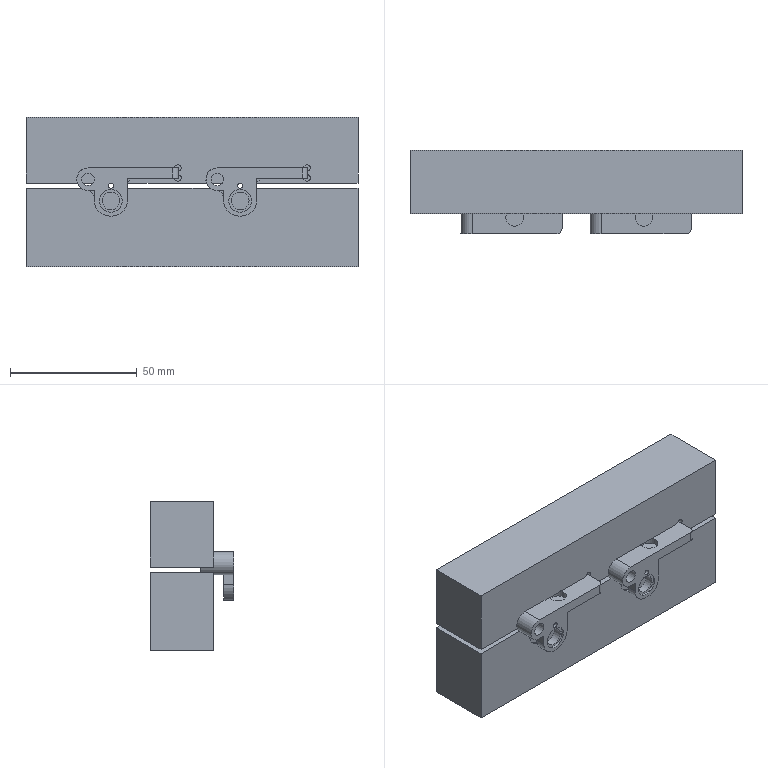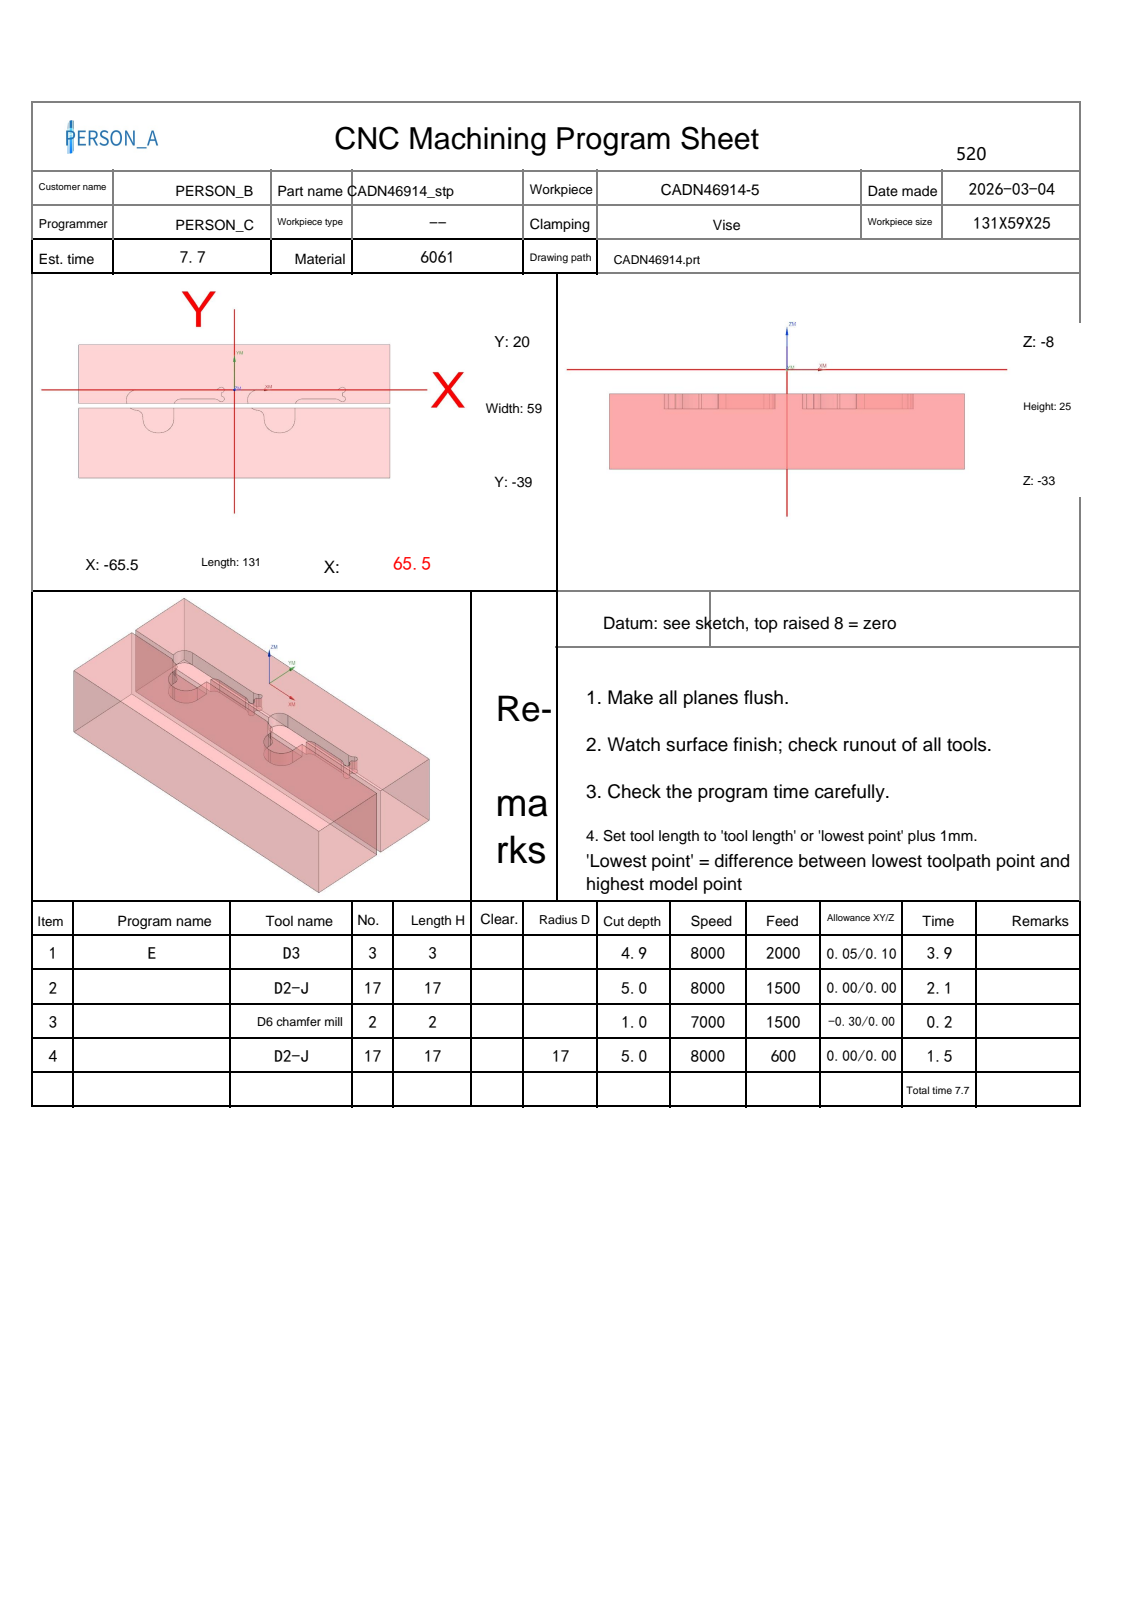NC program | NX | posted by the shop | part box 131 x 33 x 59 mm
Lines 4412 to 5424 of 10523:
N2 T17 M06
(D2-J  D=2. R=0. H=17 ce=0.00 di=0.00)
G00 G90 G54 X43.493 Y-2.917 M03 S8000
G43 H17 Z40.
M08
Z-7.9
G01 X43.492 Y-2.919 Z-7.93 F800.
Y-2.927 Z-7.958
Y-2.938 Z-7.982
Y-2.953 Z-8.004
X43.493 Y-2.971 Z-8.023
X43.496 Y-2.991 Z-8.04
X43.5 Y-3.013 Z-8.054
X43.506 Y-3.035 Z-8.066
X43.514 Y-3.058 Z-8.076
X43.524 Y-3.081 Z-8.084
X43.538 Y-3.102 Z-8.09
X43.554 Y-3.122 Z-8.095
X43.575 Y-3.139 Z-8.098
X43.599 Y-3.154 Z-8.099
X43.627 Y-3.165 Z-8.1
G02 X45.323 Y-4.176 I-1.138 J-3.835
G01 X45.5 Y-4.25
G03 X45.75 Y-4. I0.0 J.25
X45.5 Y-3.75 I-.25 J0.0
G02 X44.5 Y-2.75 I0.0 J1.
G01 Y-2.524
X44.491 Y-2.492 Z-8.101
X44.466 Y-2.471 Z-8.102
X44.428 Y-2.459 Z-8.105
X44.379 Y-2.456 Z-8.108
X44.322 Y-2.46 Z-8.112
X44.26 Y-2.472 Z-8.117
X44.195 Y-2.488 Z-8.122
X44.131 Y-2.509 Z-8.127
X44.012 Y-2.562 Z-8.138
X43.904 Y-2.63 Z-8.15
X43.807 Y-2.713 Z-8.162
X43.721 Y-2.811 Z-8.173
X43.682 Y-2.866 Z-8.178
X43.647 Y-2.922 Z-8.183
X43.619 Y-2.978 Z-8.188
X43.598 Y-3.031 Z-8.192
X43.586 Y-3.078 Z-8.195
Y-3.118 Z-8.198
X43.599 Y-3.148 Z-8.199
X43.627 Y-3.165 Z-8.2
G02 X45.323 Y-4.176 I-1.138 J-3.835
G01 X45.5 Y-4.25
G03 X45.75 Y-4. I0.0 J.25
X45.5 Y-3.75 I-.25 J0.0
G02 X44.5 Y-2.75 I0.0 J1.
G01 Y-2.524
X44.491 Y-2.492 Z-8.201
X44.466 Y-2.471 Z-8.202
X44.428 Y-2.459 Z-8.205
X44.379 Y-2.456 Z-8.208
X44.322 Y-2.46 Z-8.212
X44.26 Y-2.472 Z-8.217
X44.195 Y-2.488 Z-8.222
X44.131 Y-2.509 Z-8.227
X44.012 Y-2.562 Z-8.238
X43.904 Y-2.63 Z-8.25
X43.807 Y-2.713 Z-8.262
X43.721 Y-2.811 Z-8.273
X43.682 Y-2.866 Z-8.278
X43.647 Y-2.922 Z-8.283
X43.619 Y-2.978 Z-8.288
X43.598 Y-3.031 Z-8.292
X43.586 Y-3.078 Z-8.295
Y-3.118 Z-8.298
X43.599 Y-3.148 Z-8.299
X43.627 Y-3.165 Z-8.3
G02 X45.323 Y-4.176 I-1.138 J-3.835
G01 X45.5 Y-4.25
G03 X45.75 Y-4. I0.0 J.25
X45.5 Y-3.75 I-.25 J0.0
G02 X44.5 Y-2.75 I0.0 J1.
G01 Y-2.524
X44.491 Y-2.492 Z-8.301
X44.466 Y-2.471 Z-8.302
X44.428 Y-2.459 Z-8.305
X44.379 Y-2.456 Z-8.308
X44.322 Y-2.46 Z-8.312
X44.26 Y-2.472 Z-8.317
X44.195 Y-2.488 Z-8.322
X44.131 Y-2.509 Z-8.327
X44.012 Y-2.562 Z-8.338
X43.904 Y-2.63 Z-8.35
X43.807 Y-2.713 Z-8.362
X43.721 Y-2.811 Z-8.373
X43.682 Y-2.866 Z-8.378
X43.647 Y-2.922 Z-8.383
X43.619 Y-2.978 Z-8.388
X43.598 Y-3.031 Z-8.392
X43.586 Y-3.078 Z-8.395
Y-3.118 Z-8.398
X43.599 Y-3.148 Z-8.399
X43.627 Y-3.165 Z-8.4
G02 X45.323 Y-4.176 I-1.138 J-3.835
G01 X45.5 Y-4.25
G03 X45.75 Y-4. I0.0 J.25
X45.5 Y-3.75 I-.25 J0.0
G02 X44.5 Y-2.75 I0.0 J1.
G01 Y-2.524
X44.491 Y-2.492 Z-8.401
X44.466 Y-2.471 Z-8.402
X44.428 Y-2.459 Z-8.405
X44.379 Y-2.456 Z-8.408
X44.322 Y-2.46 Z-8.412
X44.26 Y-2.472 Z-8.417
X44.195 Y-2.488 Z-8.422
X44.131 Y-2.509 Z-8.427
X44.012 Y-2.562 Z-8.438
X43.904 Y-2.63 Z-8.45
X43.807 Y-2.713 Z-8.462
X43.721 Y-2.811 Z-8.473
X43.682 Y-2.866 Z-8.478
X43.647 Y-2.922 Z-8.483
X43.619 Y-2.978 Z-8.488
X43.598 Y-3.031 Z-8.492
X43.586 Y-3.078 Z-8.495
Y-3.118 Z-8.498
X43.599 Y-3.148 Z-8.499
X43.627 Y-3.165 Z-8.5
G02 X45.323 Y-4.176 I-1.138 J-3.835
G01 X45.5 Y-4.25
G03 X45.75 Y-4. I0.0 J.25
X45.5 Y-3.75 I-.25 J0.0
G02 X44.5 Y-2.75 I0.0 J1.
G01 Y-2.524
X44.491 Y-2.492 Z-8.501
X44.466 Y-2.471 Z-8.502
X44.428 Y-2.459 Z-8.505
X44.379 Y-2.456 Z-8.508
X44.322 Y-2.46 Z-8.512
X44.26 Y-2.472 Z-8.517
X44.195 Y-2.488 Z-8.522
X44.131 Y-2.509 Z-8.527
X44.012 Y-2.562 Z-8.538
X43.904 Y-2.63 Z-8.55
X43.807 Y-2.713 Z-8.562
X43.721 Y-2.811 Z-8.573
X43.682 Y-2.866 Z-8.578
X43.647 Y-2.922 Z-8.583
X43.619 Y-2.978 Z-8.588
X43.598 Y-3.031 Z-8.592
X43.586 Y-3.078 Z-8.595
Y-3.118 Z-8.598
X43.599 Y-3.148 Z-8.599
X43.627 Y-3.165 Z-8.6
G02 X45.323 Y-4.176 I-1.138 J-3.835
G01 X45.5 Y-4.25
G03 X45.75 Y-4. I0.0 J.25
X45.5 Y-3.75 I-.25 J0.0
G02 X44.5 Y-2.75 I0.0 J1.
G01 Y-2.524
X44.491 Y-2.492 Z-8.601
X44.466 Y-2.471 Z-8.602
X44.428 Y-2.459 Z-8.605
X44.379 Y-2.456 Z-8.608
X44.322 Y-2.46 Z-8.612
X44.26 Y-2.472 Z-8.617
X44.195 Y-2.488 Z-8.622
X44.131 Y-2.509 Z-8.627
X44.012 Y-2.562 Z-8.638
X43.904 Y-2.63 Z-8.65
X43.807 Y-2.713 Z-8.662
X43.721 Y-2.811 Z-8.673
X43.682 Y-2.866 Z-8.678
X43.647 Y-2.922 Z-8.683
X43.619 Y-2.978 Z-8.688
X43.598 Y-3.031 Z-8.692
X43.586 Y-3.078 Z-8.695
Y-3.118 Z-8.698
X43.599 Y-3.148 Z-8.699
X43.627 Y-3.165 Z-8.7
G02 X45.323 Y-4.176 I-1.138 J-3.835
G01 X45.5 Y-4.25
G03 X45.75 Y-4. I0.0 J.25
X45.5 Y-3.75 I-.25 J0.0
G02 X44.5 Y-2.75 I0.0 J1.
G01 Y-2.524
X44.491 Y-2.492 Z-8.701
X44.466 Y-2.471 Z-8.702
X44.428 Y-2.459 Z-8.705
X44.379 Y-2.456 Z-8.708
X44.322 Y-2.46 Z-8.712
X44.26 Y-2.472 Z-8.717
X44.195 Y-2.488 Z-8.722
X44.131 Y-2.509 Z-8.727
X44.012 Y-2.562 Z-8.738
X43.904 Y-2.63 Z-8.75
X43.807 Y-2.713 Z-8.762
X43.721 Y-2.811 Z-8.773
X43.682 Y-2.866 Z-8.778
X43.647 Y-2.922 Z-8.783
X43.619 Y-2.978 Z-8.788
X43.598 Y-3.031 Z-8.792
X43.586 Y-3.078 Z-8.795
Y-3.118 Z-8.798
X43.599 Y-3.148 Z-8.799
X43.627 Y-3.165 Z-8.8
G02 X45.323 Y-4.176 I-1.138 J-3.835
G01 X45.5 Y-4.25
G03 X45.75 Y-4. I0.0 J.25
X45.5 Y-3.75 I-.25 J0.0
G02 X44.5 Y-2.75 I0.0 J1.
G01 Y-2.524
X44.491 Y-2.492 Z-8.801
X44.466 Y-2.471 Z-8.802
X44.428 Y-2.459 Z-8.805
X44.379 Y-2.456 Z-8.808
X44.322 Y-2.46 Z-8.812
X44.26 Y-2.472 Z-8.817
X44.195 Y-2.488 Z-8.822
X44.131 Y-2.509 Z-8.827
X44.012 Y-2.562 Z-8.838
X43.904 Y-2.63 Z-8.85
X43.807 Y-2.713 Z-8.862
X43.721 Y-2.811 Z-8.873
X43.682 Y-2.866 Z-8.878
X43.647 Y-2.922 Z-8.883
X43.619 Y-2.978 Z-8.888
X43.598 Y-3.031 Z-8.892
X43.586 Y-3.078 Z-8.895
Y-3.118 Z-8.898
X43.599 Y-3.148 Z-8.899
X43.627 Y-3.165 Z-8.9
G02 X45.323 Y-4.176 I-1.138 J-3.835
G01 X45.5 Y-4.25
G03 X45.75 Y-4. I0.0 J.25
X45.5 Y-3.75 I-.25 J0.0
G02 X44.5 Y-2.75 I0.0 J1.
G01 Y-2.524
X44.491 Y-2.492 Z-8.901
X44.466 Y-2.471 Z-8.902
X44.428 Y-2.459 Z-8.905
X44.379 Y-2.456 Z-8.908
X44.322 Y-2.46 Z-8.912
X44.26 Y-2.472 Z-8.917
X44.195 Y-2.488 Z-8.922
X44.131 Y-2.509 Z-8.927
X44.012 Y-2.562 Z-8.938
X43.904 Y-2.63 Z-8.95
X43.807 Y-2.713 Z-8.962
X43.721 Y-2.811 Z-8.973
X43.682 Y-2.866 Z-8.978
X43.647 Y-2.922 Z-8.983
X43.619 Y-2.978 Z-8.988
X43.598 Y-3.031 Z-8.992
X43.586 Y-3.078 Z-8.995
Y-3.118 Z-8.998
X43.599 Y-3.148 Z-8.999
X43.627 Y-3.165 Z-9.
G02 X45.323 Y-4.176 I-1.138 J-3.835
G01 X45.5 Y-4.25
G03 X45.75 Y-4. I0.0 J.25
X45.5 Y-3.75 I-.25 J0.0
G02 X44.5 Y-2.75 I0.0 J1.
G01 Y-2.524
X44.491 Y-2.492 Z-9.001
X44.466 Y-2.471 Z-9.002
X44.428 Y-2.459 Z-9.005
X44.379 Y-2.456 Z-9.008
X44.322 Y-2.46 Z-9.012
X44.26 Y-2.472 Z-9.017
X44.195 Y-2.488 Z-9.022
X44.131 Y-2.509 Z-9.027
X44.012 Y-2.562 Z-9.038
X43.904 Y-2.63 Z-9.05
X43.807 Y-2.713 Z-9.062
X43.721 Y-2.811 Z-9.073
X43.682 Y-2.866 Z-9.078
X43.647 Y-2.922 Z-9.083
X43.619 Y-2.978 Z-9.088
X43.598 Y-3.031 Z-9.092
X43.586 Y-3.078 Z-9.095
Y-3.118 Z-9.098
X43.599 Y-3.148 Z-9.099
X43.627 Y-3.165 Z-9.1
G02 X45.323 Y-4.176 I-1.138 J-3.835
G01 X45.5 Y-4.25
G03 X45.75 Y-4. I0.0 J.25
X45.5 Y-3.75 I-.25 J0.0
G02 X44.5 Y-2.75 I0.0 J1.
G01 Y-2.524
X44.491 Y-2.492 Z-9.101
X44.466 Y-2.471 Z-9.102
X44.428 Y-2.459 Z-9.105
X44.379 Y-2.456 Z-9.108
X44.322 Y-2.46 Z-9.112
X44.26 Y-2.472 Z-9.117
X44.195 Y-2.488 Z-9.122
X44.131 Y-2.509 Z-9.127
X44.012 Y-2.562 Z-9.138
X43.904 Y-2.63 Z-9.15
X43.807 Y-2.713 Z-9.162
X43.721 Y-2.811 Z-9.173
X43.682 Y-2.866 Z-9.178
X43.647 Y-2.922 Z-9.183
X43.619 Y-2.978 Z-9.188
X43.598 Y-3.031 Z-9.192
X43.586 Y-3.078 Z-9.195
Y-3.118 Z-9.198
X43.599 Y-3.148 Z-9.199
X43.627 Y-3.165 Z-9.2
G02 X45.323 Y-4.176 I-1.138 J-3.835
G01 X45.5 Y-4.25
G03 X45.75 Y-4. I0.0 J.25
X45.5 Y-3.75 I-.25 J0.0
G02 X44.5 Y-2.75 I0.0 J1.
G01 Y-2.524
X44.491 Y-2.492 Z-9.201
X44.466 Y-2.471 Z-9.202
X44.428 Y-2.459 Z-9.205
X44.379 Y-2.456 Z-9.208
X44.322 Y-2.46 Z-9.212
X44.26 Y-2.472 Z-9.217
X44.195 Y-2.488 Z-9.222
X44.131 Y-2.509 Z-9.227
X44.012 Y-2.562 Z-9.238
X43.904 Y-2.63 Z-9.25
X43.807 Y-2.713 Z-9.262
X43.721 Y-2.811 Z-9.273
X43.682 Y-2.866 Z-9.278
X43.647 Y-2.922 Z-9.283
X43.619 Y-2.978 Z-9.288
X43.598 Y-3.031 Z-9.292
X43.586 Y-3.078 Z-9.295
Y-3.118 Z-9.298
X43.599 Y-3.148 Z-9.299
X43.627 Y-3.165 Z-9.3
G02 X45.323 Y-4.176 I-1.138 J-3.835
G01 X45.5 Y-4.25
G03 X45.75 Y-4. I0.0 J.25
X45.5 Y-3.75 I-.25 J0.0
G02 X44.5 Y-2.75 I0.0 J1.
G01 Y-2.524
X44.491 Y-2.492 Z-9.301
X44.466 Y-2.471 Z-9.302
X44.428 Y-2.459 Z-9.305
X44.379 Y-2.456 Z-9.308
X44.322 Y-2.46 Z-9.312
X44.26 Y-2.472 Z-9.317
X44.195 Y-2.488 Z-9.322
X44.131 Y-2.509 Z-9.327
X44.012 Y-2.562 Z-9.338
X43.904 Y-2.63 Z-9.35
X43.807 Y-2.713 Z-9.362
X43.721 Y-2.811 Z-9.373
X43.682 Y-2.866 Z-9.378
X43.647 Y-2.922 Z-9.383
X43.619 Y-2.978 Z-9.388
X43.598 Y-3.031 Z-9.392
X43.586 Y-3.078 Z-9.395
Y-3.118 Z-9.398
X43.599 Y-3.148 Z-9.399
X43.627 Y-3.165 Z-9.4
G02 X45.323 Y-4.176 I-1.138 J-3.835
G01 X45.5 Y-4.25
G03 X45.75 Y-4. I0.0 J.25
X45.5 Y-3.75 I-.25 J0.0
G02 X44.5 Y-2.75 I0.0 J1.
G01 Y-2.524
X44.491 Y-2.492 Z-9.401
X44.466 Y-2.471 Z-9.402
X44.428 Y-2.459 Z-9.405
X44.379 Y-2.456 Z-9.408
X44.322 Y-2.46 Z-9.412
X44.26 Y-2.472 Z-9.417
X44.195 Y-2.488 Z-9.422
X44.131 Y-2.509 Z-9.427
X44.012 Y-2.562 Z-9.438
X43.904 Y-2.63 Z-9.45
X43.807 Y-2.713 Z-9.462
X43.721 Y-2.811 Z-9.473
X43.682 Y-2.866 Z-9.478
X43.647 Y-2.922 Z-9.483
X43.619 Y-2.978 Z-9.488
X43.598 Y-3.031 Z-9.492
X43.586 Y-3.078 Z-9.495
Y-3.118 Z-9.498
X43.599 Y-3.148 Z-9.499
X43.627 Y-3.165 Z-9.5
G02 X45.323 Y-4.176 I-1.138 J-3.835
G01 X45.5 Y-4.25
G03 X45.75 Y-4. I0.0 J.25
X45.5 Y-3.75 I-.25 J0.0
G02 X44.5 Y-2.75 I0.0 J1.
G01 Y-2.524
X44.491 Y-2.492 Z-9.501
X44.466 Y-2.471 Z-9.502
X44.428 Y-2.459 Z-9.505
X44.379 Y-2.456 Z-9.508
X44.322 Y-2.46 Z-9.512
X44.26 Y-2.472 Z-9.517
X44.195 Y-2.488 Z-9.522
X44.131 Y-2.509 Z-9.527
X44.012 Y-2.562 Z-9.538
X43.904 Y-2.63 Z-9.55
X43.807 Y-2.713 Z-9.562
X43.721 Y-2.811 Z-9.573
X43.682 Y-2.866 Z-9.578
X43.647 Y-2.922 Z-9.583
X43.619 Y-2.978 Z-9.588
X43.598 Y-3.031 Z-9.592
X43.586 Y-3.078 Z-9.595
Y-3.118 Z-9.598
X43.599 Y-3.148 Z-9.599
X43.627 Y-3.165 Z-9.6
G02 X45.323 Y-4.176 I-1.138 J-3.835
G01 X45.5 Y-4.25
G03 X45.75 Y-4. I0.0 J.25
X45.5 Y-3.75 I-.25 J0.0
G02 X44.5 Y-2.75 I0.0 J1.
G01 Y-2.524
X44.491 Y-2.492 Z-9.601
X44.466 Y-2.471 Z-9.602
X44.428 Y-2.459 Z-9.605
X44.379 Y-2.456 Z-9.608
X44.322 Y-2.46 Z-9.612
X44.26 Y-2.472 Z-9.617
X44.195 Y-2.488 Z-9.622
X44.131 Y-2.509 Z-9.627
X44.012 Y-2.562 Z-9.638
X43.904 Y-2.63 Z-9.65
X43.807 Y-2.713 Z-9.662
X43.721 Y-2.811 Z-9.673
X43.682 Y-2.866 Z-9.678
X43.647 Y-2.922 Z-9.683
X43.619 Y-2.978 Z-9.688
X43.598 Y-3.031 Z-9.692
X43.586 Y-3.078 Z-9.695
Y-3.118 Z-9.698
X43.599 Y-3.148 Z-9.699
X43.627 Y-3.165 Z-9.7
G02 X45.323 Y-4.176 I-1.138 J-3.835
G01 X45.5 Y-4.25
G03 X45.75 Y-4. I0.0 J.25
X45.5 Y-3.75 I-.25 J0.0
G02 X44.5 Y-2.75 I0.0 J1.
G01 Y-2.524
X44.491 Y-2.492 Z-9.701
X44.466 Y-2.471 Z-9.702
X44.428 Y-2.459 Z-9.705
X44.379 Y-2.456 Z-9.708
X44.322 Y-2.46 Z-9.712
X44.26 Y-2.472 Z-9.717
X44.195 Y-2.488 Z-9.722
X44.131 Y-2.509 Z-9.727
X44.012 Y-2.562 Z-9.738
X43.904 Y-2.63 Z-9.75
X43.807 Y-2.713 Z-9.762
X43.721 Y-2.811 Z-9.773
X43.682 Y-2.866 Z-9.778
X43.647 Y-2.922 Z-9.783
X43.619 Y-2.978 Z-9.788
X43.598 Y-3.031 Z-9.792
X43.586 Y-3.078 Z-9.795
Y-3.118 Z-9.798
X43.599 Y-3.148 Z-9.799
X43.627 Y-3.165 Z-9.8
G02 X45.323 Y-4.176 I-1.138 J-3.835
G01 X45.5 Y-4.25
G03 X45.75 Y-4. I0.0 J.25
X45.5 Y-3.75 I-.25 J0.0
G02 X44.5 Y-2.75 I0.0 J1.
G01 Y-2.524
X44.491 Y-2.492 Z-9.801
X44.466 Y-2.471 Z-9.802
X44.428 Y-2.459 Z-9.805
X44.379 Y-2.456 Z-9.808
X44.322 Y-2.46 Z-9.812
X44.26 Y-2.472 Z-9.817
X44.195 Y-2.488 Z-9.822
X44.131 Y-2.509 Z-9.827
X44.012 Y-2.562 Z-9.838
X43.904 Y-2.63 Z-9.85
X43.807 Y-2.713 Z-9.862
X43.721 Y-2.811 Z-9.873
X43.682 Y-2.866 Z-9.878
X43.647 Y-2.922 Z-9.883
X43.619 Y-2.978 Z-9.888
X43.598 Y-3.031 Z-9.892
X43.586 Y-3.078 Z-9.895
Y-3.118 Z-9.898
X43.599 Y-3.148 Z-9.899
X43.627 Y-3.165 Z-9.9
G02 X45.323 Y-4.176 I-1.138 J-3.835
G01 X45.5 Y-4.25
G03 X45.75 Y-4. I0.0 J.25
X45.5 Y-3.75 I-.25 J0.0
G02 X44.5 Y-2.75 I0.0 J1.
G01 Y-2.524
X44.491 Y-2.492 Z-9.901
X44.466 Y-2.471 Z-9.902
X44.428 Y-2.459 Z-9.905
X44.379 Y-2.456 Z-9.908
X44.322 Y-2.46 Z-9.912
X44.26 Y-2.472 Z-9.917
X44.195 Y-2.488 Z-9.922
X44.131 Y-2.509 Z-9.927
X44.012 Y-2.562 Z-9.938
X43.904 Y-2.63 Z-9.95
X43.807 Y-2.713 Z-9.962
X43.721 Y-2.811 Z-9.973
X43.682 Y-2.866 Z-9.978
X43.647 Y-2.922 Z-9.983
X43.619 Y-2.978 Z-9.988
X43.598 Y-3.031 Z-9.992
X43.586 Y-3.078 Z-9.995
Y-3.118 Z-9.998
X43.599 Y-3.148 Z-9.999
X43.627 Y-3.165 Z-10.
G02 X45.323 Y-4.176 I-1.138 J-3.835
G01 X45.5 Y-4.25
G03 X45.75 Y-4. I0.0 J.25
X45.5 Y-3.75 I-.25 J0.0
G02 X44.5 Y-2.75 I0.0 J1.
G01 Y-2.524
X44.491 Y-2.492 Z-10.001
X44.466 Y-2.471 Z-10.002
X44.428 Y-2.459 Z-10.005
X44.379 Y-2.456 Z-10.008
X44.322 Y-2.46 Z-10.012
X44.26 Y-2.472 Z-10.017
X44.195 Y-2.488 Z-10.022
X44.131 Y-2.509 Z-10.027
X44.012 Y-2.562 Z-10.038
X43.904 Y-2.63 Z-10.05
X43.807 Y-2.713 Z-10.062
X43.721 Y-2.811 Z-10.073
X43.682 Y-2.866 Z-10.078
X43.647 Y-2.922 Z-10.083
X43.619 Y-2.978 Z-10.088
X43.598 Y-3.031 Z-10.092
X43.586 Y-3.078 Z-10.095
Y-3.118 Z-10.098
X43.599 Y-3.148 Z-10.099
X43.627 Y-3.165 Z-10.1
G02 X45.323 Y-4.176 I-1.138 J-3.835
G01 X45.5 Y-4.25
G03 X45.75 Y-4. I0.0 J.25
X45.5 Y-3.75 I-.25 J0.0
G02 X44.5 Y-2.75 I0.0 J1.
G01 Y-2.524
X44.491 Y-2.492 Z-10.101
X44.466 Y-2.471 Z-10.102
X44.428 Y-2.459 Z-10.105
X44.379 Y-2.456 Z-10.108
X44.322 Y-2.46 Z-10.112
X44.26 Y-2.472 Z-10.117
X44.195 Y-2.488 Z-10.122
X44.131 Y-2.509 Z-10.127
X44.012 Y-2.562 Z-10.138
X43.904 Y-2.63 Z-10.15
X43.807 Y-2.713 Z-10.162
X43.721 Y-2.811 Z-10.173
X43.682 Y-2.866 Z-10.178
X43.647 Y-2.922 Z-10.183
X43.619 Y-2.978 Z-10.188
X43.598 Y-3.031 Z-10.192
X43.586 Y-3.078 Z-10.195
Y-3.118 Z-10.198
X43.599 Y-3.148 Z-10.199
X43.627 Y-3.165 Z-10.2
G02 X45.323 Y-4.176 I-1.138 J-3.835
G01 X45.5 Y-4.25
G03 X45.75 Y-4. I0.0 J.25
X45.5 Y-3.75 I-.25 J0.0
G02 X44.5 Y-2.75 I0.0 J1.
G01 Y-2.524
X44.491 Y-2.492 Z-10.201
X44.466 Y-2.471 Z-10.202
X44.428 Y-2.459 Z-10.205
X44.379 Y-2.456 Z-10.208
X44.322 Y-2.46 Z-10.212
X44.26 Y-2.472 Z-10.217
X44.195 Y-2.488 Z-10.222
X44.131 Y-2.509 Z-10.227
X44.012 Y-2.562 Z-10.238
X43.904 Y-2.63 Z-10.25
X43.807 Y-2.713 Z-10.262
X43.721 Y-2.811 Z-10.273
X43.682 Y-2.866 Z-10.278
X43.647 Y-2.922 Z-10.283
X43.619 Y-2.978 Z-10.288
X43.598 Y-3.031 Z-10.292
X43.586 Y-3.078 Z-10.295
Y-3.118 Z-10.298
X43.599 Y-3.148 Z-10.299
X43.627 Y-3.165 Z-10.3
G02 X45.323 Y-4.176 I-1.138 J-3.835
G01 X45.5 Y-4.25
G03 X45.75 Y-4. I0.0 J.25
X45.5 Y-3.75 I-.25 J0.0
G02 X44.5 Y-2.75 I0.0 J1.
G01 Y-2.524
X44.491 Y-2.492 Z-10.301
X44.466 Y-2.471 Z-10.302
X44.428 Y-2.459 Z-10.305
X44.379 Y-2.456 Z-10.308
X44.322 Y-2.46 Z-10.312
X44.26 Y-2.472 Z-10.317
X44.195 Y-2.488 Z-10.322
X44.131 Y-2.509 Z-10.327
X44.012 Y-2.562 Z-10.338
X43.904 Y-2.63 Z-10.35
X43.807 Y-2.713 Z-10.362
X43.721 Y-2.811 Z-10.373
X43.682 Y-2.866 Z-10.378
X43.647 Y-2.922 Z-10.383
X43.619 Y-2.978 Z-10.388
X43.598 Y-3.031 Z-10.392
X43.586 Y-3.078 Z-10.395
Y-3.118 Z-10.398
X43.599 Y-3.148 Z-10.399
X43.627 Y-3.165 Z-10.4
G02 X45.323 Y-4.176 I-1.138 J-3.835
G01 X45.5 Y-4.25
G03 X45.75 Y-4. I0.0 J.25
X45.5 Y-3.75 I-.25 J0.0
G02 X44.5 Y-2.75 I0.0 J1.
G01 Y-2.524
X44.491 Y-2.492 Z-10.401
X44.466 Y-2.471 Z-10.402
X44.428 Y-2.459 Z-10.405
X44.379 Y-2.456 Z-10.408
X44.322 Y-2.46 Z-10.412
X44.26 Y-2.472 Z-10.417
X44.195 Y-2.488 Z-10.422
X44.131 Y-2.509 Z-10.427
X44.012 Y-2.562 Z-10.438
X43.904 Y-2.63 Z-10.45
X43.807 Y-2.713 Z-10.462
X43.721 Y-2.811 Z-10.473
X43.682 Y-2.866 Z-10.478
X43.647 Y-2.922 Z-10.483
X43.619 Y-2.978 Z-10.488
X43.598 Y-3.031 Z-10.492
X43.586 Y-3.078 Z-10.495
Y-3.118 Z-10.498
X43.599 Y-3.148 Z-10.499
X43.627 Y-3.165 Z-10.5
G02 X45.323 Y-4.176 I-1.138 J-3.835
G01 X45.5 Y-4.25
G03 X45.75 Y-4. I0.0 J.25
X45.5 Y-3.75 I-.25 J0.0
G02 X44.5 Y-2.75 I0.0 J1.
G01 Y-2.524
X44.491 Y-2.492 Z-10.501
X44.466 Y-2.471 Z-10.502
X44.428 Y-2.459 Z-10.505
X44.379 Y-2.456 Z-10.508
X44.322 Y-2.46 Z-10.512
X44.26 Y-2.472 Z-10.517
X44.195 Y-2.488 Z-10.522
X44.131 Y-2.509 Z-10.527
X44.012 Y-2.562 Z-10.538
X43.904 Y-2.63 Z-10.55
X43.807 Y-2.713 Z-10.562
X43.721 Y-2.811 Z-10.573
X43.682 Y-2.866 Z-10.578
X43.647 Y-2.922 Z-10.583
X43.619 Y-2.978 Z-10.588
X43.598 Y-3.031 Z-10.592
X43.586 Y-3.078 Z-10.595
Y-3.118 Z-10.598
X43.599 Y-3.148 Z-10.599
X43.627 Y-3.165 Z-10.6
G02 X45.323 Y-4.176 I-1.138 J-3.835
G01 X45.5 Y-4.25
G03 X45.75 Y-4. I0.0 J.25
X45.5 Y-3.75 I-.25 J0.0
G02 X44.5 Y-2.75 I0.0 J1.
G01 Y-2.524
X44.491 Y-2.492 Z-10.601
X44.466 Y-2.471 Z-10.602
X44.428 Y-2.459 Z-10.605
X44.379 Y-2.456 Z-10.608
X44.322 Y-2.46 Z-10.612
X44.26 Y-2.472 Z-10.617
X44.195 Y-2.488 Z-10.622
X44.131 Y-2.509 Z-10.627
X44.012 Y-2.562 Z-10.638
X43.904 Y-2.63 Z-10.65
X43.807 Y-2.713 Z-10.662
X43.721 Y-2.811 Z-10.673
X43.682 Y-2.866 Z-10.678
X43.647 Y-2.922 Z-10.683
X43.619 Y-2.978 Z-10.688
X43.598 Y-3.031 Z-10.692
X43.586 Y-3.078 Z-10.695
Y-3.118 Z-10.698
X43.599 Y-3.148 Z-10.699
X43.627 Y-3.165 Z-10.7
G02 X45.323 Y-4.176 I-1.138 J-3.835
G01 X45.5 Y-4.25
G03 X45.75 Y-4. I0.0 J.25
X45.5 Y-3.75 I-.25 J0.0
G02 X44.5 Y-2.75 I0.0 J1.
G01 Y-2.524
X44.491 Y-2.492 Z-10.701
X44.466 Y-2.471 Z-10.702
X44.428 Y-2.459 Z-10.705
X44.379 Y-2.456 Z-10.708
X44.322 Y-2.46 Z-10.712
X44.26 Y-2.472 Z-10.717
X44.195 Y-2.488 Z-10.722
X44.131 Y-2.509 Z-10.727
X44.012 Y-2.562 Z-10.738
X43.904 Y-2.63 Z-10.75
X43.807 Y-2.713 Z-10.762
X43.721 Y-2.811 Z-10.773
X43.682 Y-2.866 Z-10.778
X43.647 Y-2.922 Z-10.783
X43.619 Y-2.978 Z-10.788
X43.598 Y-3.031 Z-10.792
X43.586 Y-3.078 Z-10.795
Y-3.118 Z-10.798
X43.599 Y-3.148 Z-10.799
X43.627 Y-3.165 Z-10.8
G02 X45.323 Y-4.176 I-1.138 J-3.835
G01 X45.5 Y-4.25
G03 X45.75 Y-4. I0.0 J.25
X45.5 Y-3.75 I-.25 J0.0
G02 X44.5 Y-2.75 I0.0 J1.
G01 Y-2.524
X44.491 Y-2.492 Z-10.801
X44.466 Y-2.471 Z-10.802
X44.428 Y-2.459 Z-10.805
X44.379 Y-2.456 Z-10.808
X44.322 Y-2.46 Z-10.812
X44.26 Y-2.472 Z-10.817
X44.195 Y-2.488 Z-10.822
X44.131 Y-2.509 Z-10.827
X44.012 Y-2.562 Z-10.838
X43.904 Y-2.63 Z-10.85
X43.807 Y-2.713 Z-10.862
X43.721 Y-2.811 Z-10.873
X43.682 Y-2.866 Z-10.878
X43.647 Y-2.922 Z-10.883
X43.619 Y-2.978 Z-10.888
X43.598 Y-3.031 Z-10.892
X43.586 Y-3.078 Z-10.895
Y-3.118 Z-10.898
X43.599 Y-3.148 Z-10.899
X43.627 Y-3.165 Z-10.9
G02 X45.323 Y-4.176 I-1.138 J-3.835
G01 X45.5 Y-4.25
G03 X45.75 Y-4. I0.0 J.25
X45.5 Y-3.75 I-.25 J0.0
G02 X44.5 Y-2.75 I0.0 J1.
G01 Y-2.524
X44.491 Y-2.492 Z-10.901
X44.466 Y-2.471 Z-10.902
X44.428 Y-2.459 Z-10.905
X44.379 Y-2.456 Z-10.908
X44.322 Y-2.46 Z-10.912
X44.26 Y-2.472 Z-10.917
X44.195 Y-2.488 Z-10.922
X44.131 Y-2.509 Z-10.927
X44.012 Y-2.562 Z-10.938
X43.904 Y-2.63 Z-10.95
X43.807 Y-2.713 Z-10.962
X43.721 Y-2.811 Z-10.973
X43.682 Y-2.866 Z-10.978
X43.647 Y-2.922 Z-10.983
X43.619 Y-2.978 Z-10.988
X43.598 Y-3.031 Z-10.992
X43.586 Y-3.078 Z-10.995
Y-3.118 Z-10.998
X43.599 Y-3.148 Z-10.999
X43.627 Y-3.165 Z-11.
G02 X45.323 Y-4.176 I-1.138 J-3.835
G01 X45.5 Y-4.25
G03 X45.75 Y-4. I0.0 J.25
X45.5 Y-3.75 I-.25 J0.0
G02 X44.5 Y-2.75 I0.0 J1.
G01 Y-2.524
X44.491 Y-2.492 Z-11.001
X44.466 Y-2.471 Z-11.002
X44.428 Y-2.459 Z-11.005
X44.379 Y-2.456 Z-11.008
X44.322 Y-2.46 Z-11.012
X44.26 Y-2.472 Z-11.017
X44.195 Y-2.488 Z-11.022
X44.131 Y-2.509 Z-11.027
X44.012 Y-2.562 Z-11.038
X43.904 Y-2.63 Z-11.05
X43.807 Y-2.713 Z-11.062
X43.721 Y-2.811 Z-11.073
X43.682 Y-2.866 Z-11.078
X43.647 Y-2.922 Z-11.083
X43.619 Y-2.978 Z-11.088
X43.598 Y-3.031 Z-11.092
X43.586 Y-3.078 Z-11.095
Y-3.118 Z-11.098
X43.599 Y-3.148 Z-11.099
X43.627 Y-3.165 Z-11.1
G02 X45.323 Y-4.176 I-1.138 J-3.835
G01 X45.5 Y-4.25
G03 X45.75 Y-4. I0.0 J.25
X45.5 Y-3.75 I-.25 J0.0
G02 X44.5 Y-2.75 I0.0 J1.
G01 Y-2.524
X44.491 Y-2.492 Z-11.101
X44.466 Y-2.471 Z-11.102
X44.428 Y-2.459 Z-11.105
X44.379 Y-2.456 Z-11.108
X44.322 Y-2.46 Z-11.112
X44.26 Y-2.472 Z-11.117
X44.195 Y-2.488 Z-11.122
X44.131 Y-2.509 Z-11.127
X44.012 Y-2.562 Z-11.138
X43.904 Y-2.63 Z-11.15
X43.807 Y-2.713 Z-11.162
X43.721 Y-2.811 Z-11.173
X43.682 Y-2.866 Z-11.178
X43.647 Y-2.922 Z-11.183
X43.619 Y-2.978 Z-11.188
X43.598 Y-3.031 Z-11.192
X43.586 Y-3.078 Z-11.195
Y-3.118 Z-11.198
X43.599 Y-3.148 Z-11.199
X43.627 Y-3.165 Z-11.2
G02 X45.323 Y-4.176 I-1.138 J-3.835
G01 X45.5 Y-4.25
G03 X45.75 Y-4. I0.0 J.25
X45.5 Y-3.75 I-.25 J0.0
G02 X44.5 Y-2.75 I0.0 J1.
G01 Y-2.524
X44.491 Y-2.492 Z-11.201
X44.466 Y-2.471 Z-11.202
X44.428 Y-2.459 Z-11.205
X44.379 Y-2.456 Z-11.208
X44.322 Y-2.46 Z-11.212
X44.26 Y-2.472 Z-11.217
X44.195 Y-2.488 Z-11.222
X44.131 Y-2.509 Z-11.227
X44.012 Y-2.562 Z-11.238
X43.904 Y-2.63 Z-11.25
X43.807 Y-2.713 Z-11.262
X43.721 Y-2.811 Z-11.273
X43.682 Y-2.866 Z-11.278
X43.647 Y-2.922 Z-11.283
X43.619 Y-2.978 Z-11.288
X43.598 Y-3.031 Z-11.292
X43.586 Y-3.078 Z-11.295
Y-3.118 Z-11.298
X43.599 Y-3.148 Z-11.299
X43.627 Y-3.165 Z-11.3
G02 X45.323 Y-4.176 I-1.138 J-3.835
G01 X45.5 Y-4.25
G03 X45.75 Y-4. I0.0 J.25
X45.5 Y-3.75 I-.25 J0.0
G02 X44.5 Y-2.75 I0.0 J1.
G01 Y-2.524
X44.491 Y-2.492 Z-11.301
X44.466 Y-2.471 Z-11.302
X44.428 Y-2.459 Z-11.305
X44.379 Y-2.456 Z-11.308
X44.322 Y-2.46 Z-11.312
X44.26 Y-2.472 Z-11.317
X44.195 Y-2.488 Z-11.322
X44.131 Y-2.509 Z-11.327
X44.012 Y-2.562 Z-11.338
X43.904 Y-2.63 Z-11.35
X43.807 Y-2.713 Z-11.362
X43.721 Y-2.811 Z-11.373
X43.682 Y-2.866 Z-11.378
X43.647 Y-2.922 Z-11.383
X43.619 Y-2.978 Z-11.388
X43.598 Y-3.031 Z-11.392
X43.586 Y-3.078 Z-11.395
Y-3.118 Z-11.398
X43.599 Y-3.148 Z-11.399
X43.627 Y-3.165 Z-11.4
G02 X45.323 Y-4.176 I-1.138 J-3.835
G01 X45.5 Y-4.25
G03 X45.75 Y-4. I0.0 J.25
X45.5 Y-3.75 I-.25 J0.0
G02 X44.5 Y-2.75 I0.0 J1.
G01 Y-2.524
X44.491 Y-2.492 Z-11.401
X44.466 Y-2.471 Z-11.402
X44.428 Y-2.459 Z-11.405
X44.379 Y-2.456 Z-11.408
X44.322 Y-2.46 Z-11.412
X44.26 Y-2.472 Z-11.417
X44.195 Y-2.488 Z-11.422
X44.131 Y-2.509 Z-11.427
X44.012 Y-2.562 Z-11.438
X43.904 Y-2.63 Z-11.45
X43.807 Y-2.713 Z-11.462
X43.721 Y-2.811 Z-11.473
X43.682 Y-2.866 Z-11.478
X43.647 Y-2.922 Z-11.483
X43.619 Y-2.978 Z-11.488
X43.598 Y-3.031 Z-11.492
X43.586 Y-3.078 Z-11.495
Y-3.118 Z-11.498
X43.599 Y-3.148 Z-11.499
X43.627 Y-3.165 Z-11.5
G02 X45.323 Y-4.176 I-1.138 J-3.835
G01 X45.5 Y-4.25
G03 X45.75 Y-4. I0.0 J.25
X45.5 Y-3.75 I-.25 J0.0
G02 X44.5 Y-2.75 I0.0 J1.
G01 Y-2.524
X44.491 Y-2.492 Z-11.501
X44.466 Y-2.471 Z-11.502
X44.428 Y-2.459 Z-11.505
X44.379 Y-2.456 Z-11.508
X44.322 Y-2.46 Z-11.512
X44.26 Y-2.472 Z-11.517
X44.195 Y-2.488 Z-11.522
X44.131 Y-2.509 Z-11.527
X44.012 Y-2.562 Z-11.538
X43.904 Y-2.63 Z-11.55
X43.807 Y-2.713 Z-11.562
X43.721 Y-2.811 Z-11.573
X43.682 Y-2.866 Z-11.578
X43.647 Y-2.922 Z-11.583
X43.619 Y-2.978 Z-11.588
X43.598 Y-3.031 Z-11.592
X43.586 Y-3.078 Z-11.595
Y-3.118 Z-11.598
X43.599 Y-3.148 Z-11.599
X43.627 Y-3.165 Z-11.6
G02 X45.323 Y-4.176 I-1.138 J-3.835
G01 X45.5 Y-4.25
G03 X45.75 Y-4. I0.0 J.25
X45.5 Y-3.75 I-.25 J0.0
G02 X44.5 Y-2.75 I0.0 J1.
G01 Y-2.524
X44.491 Y-2.492 Z-11.601
X44.466 Y-2.471 Z-11.602
X44.428 Y-2.459 Z-11.605
X44.379 Y-2.456 Z-11.608
X44.322 Y-2.46 Z-11.612
X44.26 Y-2.472 Z-11.617
X44.195 Y-2.488 Z-11.622
X44.131 Y-2.509 Z-11.627
X44.012 Y-2.562 Z-11.638
X43.904 Y-2.63 Z-11.65
X43.807 Y-2.713 Z-11.662
X43.721 Y-2.811 Z-11.673
X43.682 Y-2.866 Z-11.678
X43.647 Y-2.922 Z-11.683
X43.619 Y-2.978 Z-11.688
X43.598 Y-3.031 Z-11.692
X43.586 Y-3.078 Z-11.695
Y-3.118 Z-11.698
X43.599 Y-3.148 Z-11.699
X43.627 Y-3.165 Z-11.7
G02 X45.323 Y-4.176 I-1.138 J-3.835
G01 X45.5 Y-4.25
G03 X45.75 Y-4. I0.0 J.25
X45.5 Y-3.75 I-.25 J0.0
G02 X44.5 Y-2.75 I0.0 J1.
G01 Y-2.524
X44.491 Y-2.492 Z-11.701
X44.466 Y-2.471 Z-11.702
X44.428 Y-2.459 Z-11.705
X44.379 Y-2.456 Z-11.708
X44.322 Y-2.46 Z-11.712
X44.26 Y-2.472 Z-11.717
X44.195 Y-2.488 Z-11.722
X44.131 Y-2.509 Z-11.727
X44.012 Y-2.562 Z-11.738
X43.904 Y-2.63 Z-11.75
X43.807 Y-2.713 Z-11.762
X43.721 Y-2.811 Z-11.773
X43.682 Y-2.866 Z-11.778
X43.647 Y-2.922 Z-11.783
X43.619 Y-2.978 Z-11.788
X43.598 Y-3.031 Z-11.792
X43.586 Y-3.078 Z-11.795
Y-3.118 Z-11.798
X43.599 Y-3.148 Z-11.799
X43.627 Y-3.165 Z-11.8
G02 X45.323 Y-4.176 I-1.138 J-3.835
G01 X45.5 Y-4.25
G03 X45.75 Y-4. I0.0 J.25
X45.5 Y-3.75 I-.25 J0.0
G02 X44.5 Y-2.75 I0.0 J1.
G01 Y-2.524
X44.491 Y-2.492 Z-11.801
X44.466 Y-2.471 Z-11.802
X44.428 Y-2.459 Z-11.805
X44.379 Y-2.456 Z-11.808
X44.322 Y-2.46 Z-11.812
X44.26 Y-2.472 Z-11.817
X44.195 Y-2.488 Z-11.822
X44.131 Y-2.509 Z-11.827
X44.012 Y-2.562 Z-11.838
X43.904 Y-2.63 Z-11.85
X43.807 Y-2.713 Z-11.862
X43.721 Y-2.811 Z-11.873
X43.682 Y-2.866 Z-11.878
X43.647 Y-2.922 Z-11.883
X43.619 Y-2.978 Z-11.888
X43.598 Y-3.031 Z-11.892
X43.586 Y-3.078 Z-11.895
Y-3.118 Z-11.898
X43.599 Y-3.148 Z-11.899
X43.627 Y-3.165 Z-11.9
G02 X45.323 Y-4.176 I-1.138 J-3.835
G01 X45.5 Y-4.25
G03 X45.75 Y-4. I0.0 J.25
X45.5 Y-3.75 I-.25 J0.0